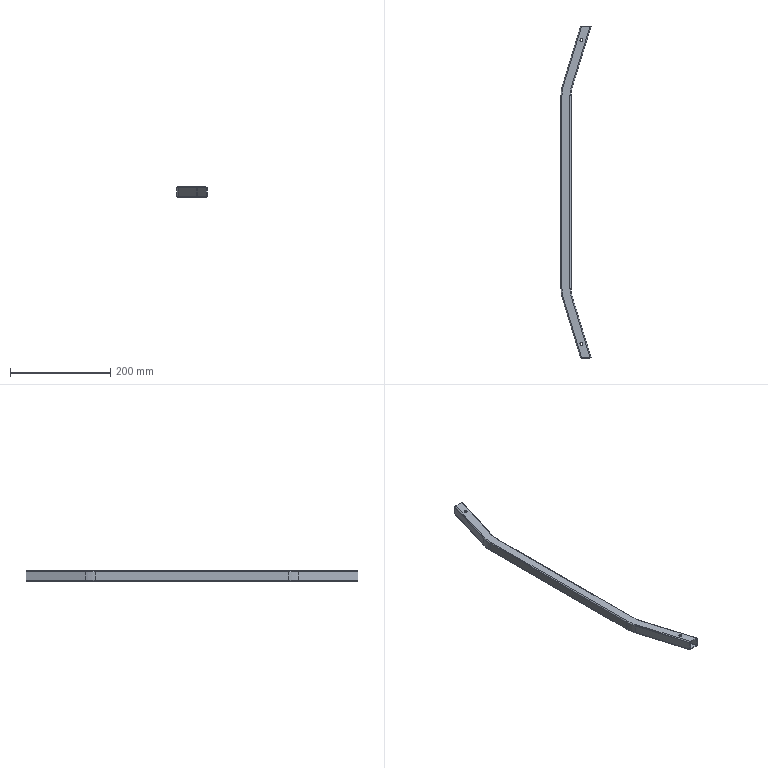Part | STEP file | 7471202 | 1 solid | 70 faces | box 59.901 x 660.964 x 20 mm | volume 72312 mm3 | cylinder 36 | plane 18 | torus 16 | commonest cylinder face diameters 1 x12 4 x12 6 x4 100 x2 103 x2 137 x2